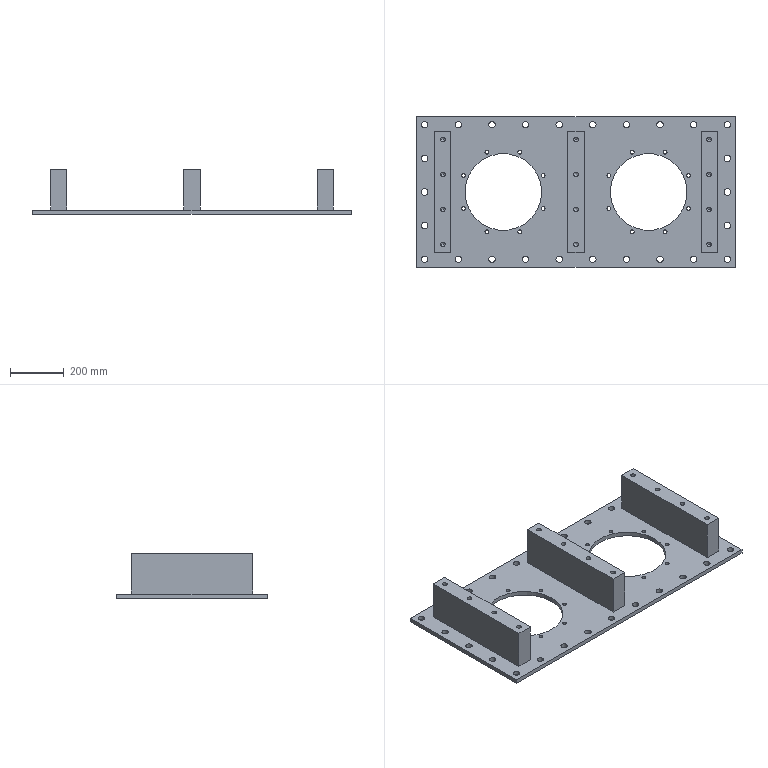Part | SolidWorks | features ICE 3, HoleWzd 2, LPattern 2, CirPattern 1, Extrusion 1, MirrorPattern 1, RefAxis 1 | 4 solids | 160 faces | box 1185 x 560 x 166 mm | volume 20349216 mm3 | cylinder 112 | cone 24 | plane 24 | commonest cylinder face diameters 24 x52 14 x32 17.5 x24 285 x4